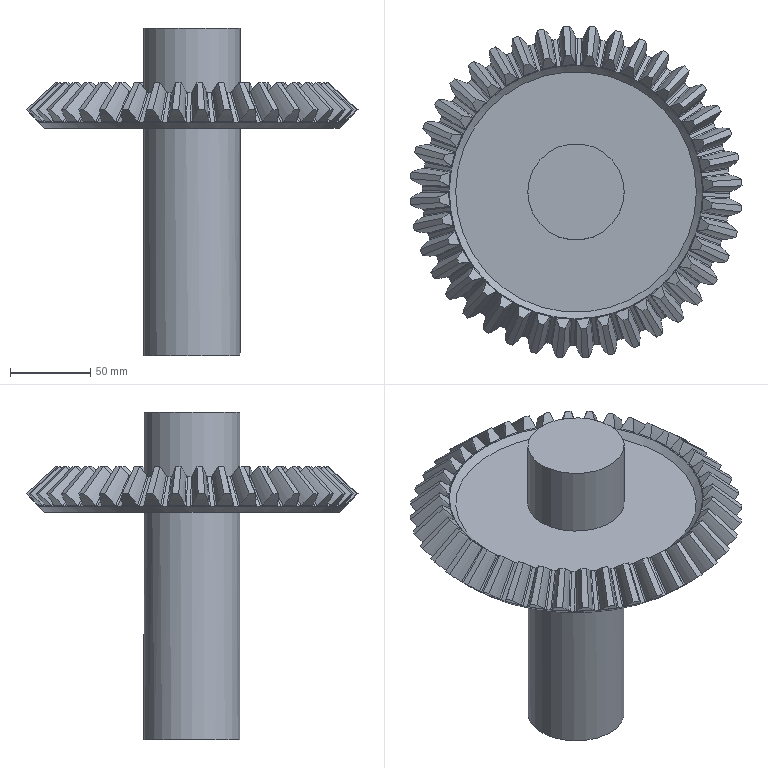Part | NX | features BREP 1 | 1 solid | 488 faces | box 206.798 x 206.798 x 204 mm | volume 1074279 mm3 | spline 320 | plane 84 | cone 82 | cylinder 2 | commonest cylinder face diameters 60 x2